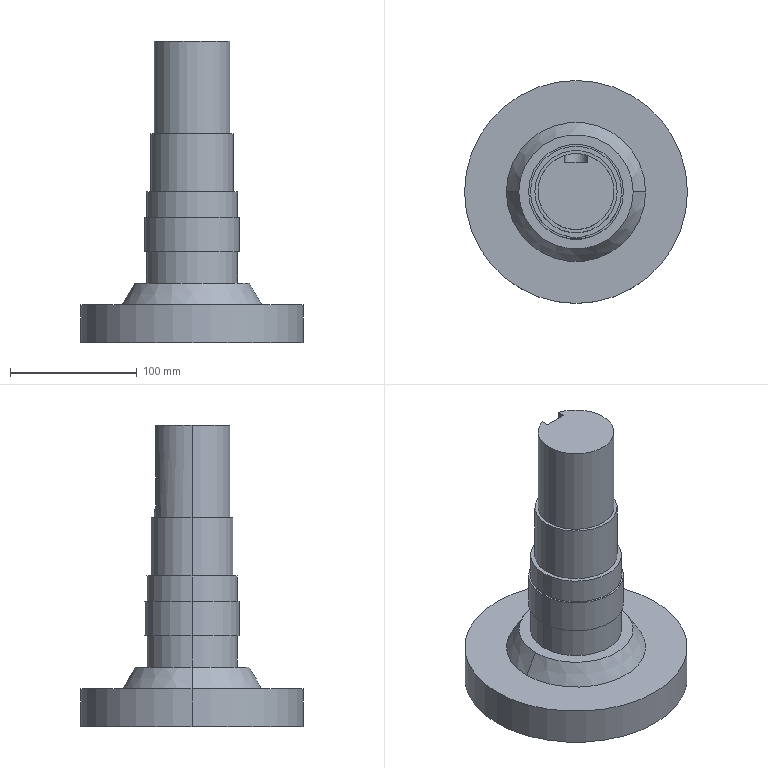Part | SolidWorks | features ICE 10, Chamfer 1, Extrusion 1, Fillet 1 | 1 solid | 37 faces | box 176 x 176 x 238 mm | volume 1296573 mm3 | cylinder 19 | plane 14 | torus 2 | cone 2 | commonest cylinder face diameters 72 x4 40 x2 60 x2 65 x2 75 x2 80 x2
STEP:
#1=CARTESIAN_POINT('',(-20.,0.,44.));
#2=VERTEX_POINT('',#1);
#3=CARTESIAN_POINT('',(20.,0.,44.));
#4=VERTEX_POINT('',#3);
#5=CARTESIAN_POINT('',(0.,0.,44.));
#6=DIRECTION('',(0.,0.,1.));
#7=DIRECTION('',(1.,0.,0.));
#8=AXIS2_PLACEMENT_3D('',#5,#6,#7);
#9=CIRCLE('',#8,20.);
#10=EDGE_CURVE('',#2,#4,#9,.T.);
#11=ORIENTED_EDGE('',*,*,#10,.T.);
#12=CARTESIAN_POINT('',(20.,0.,34.2));
#13=VERTEX_POINT('',#12);
#14=CARTESIAN_POINT('',(20.,0.,44.));
#15=DIRECTION('',(0.,0.,-1.));
#16=VECTOR('',#15,1000.);
#17=LINE('',#14,#16);
#18=EDGE_CURVE('',#4,#13,#17,.T.);
#19=ORIENTED_EDGE('',*,*,#18,.T.);
#20=CARTESIAN_POINT('',(-20.,0.,34.2));
#21=VERTEX_POINT('',#20);
#22=CARTESIAN_POINT('',(0.,0.,34.2));
#23=DIRECTION('',(0.,0.,1.));
#24=DIRECTION('',(-1.,0.,0.));
#25=AXIS2_PLACEMENT_3D('',#22,#23,#24);
#26=CIRCLE('',#25,20.);
#27=EDGE_CURVE('',#21,#13,#26,.T.);
#28=ORIENTED_EDGE('',*,*,#27,.F.);
#29=CARTESIAN_POINT('',(-20.,0.,44.));
#30=DIRECTION('',(0.,0.,-1.));
#31=VECTOR('',#30,1000.);
#32=LINE('',#29,#31);
#33=EDGE_CURVE('',#2,#21,#32,.T.);
#34=ORIENTED_EDGE('',*,*,#33,.F.);
#35=EDGE_LOOP('',(#11,#19,#28,#34));
#36=FACE_OUTER_BOUND('',#35,.T.);
#37=CARTESIAN_POINT('',(0.,0.,44.));
#38=DIRECTION('',(0.,0.,-1.));
#39=DIRECTION('',(-1.,0.,0.));
#40=AXIS2_PLACEMENT_3D('',#37,#38,#39);
#41=CYLINDRICAL_SURFACE('',#40,20.);
#42=ADVANCED_FACE('',(#36),#41,.F.);
#43=CARTESIAN_POINT('',(47.,0.,11.2));
#44=VERTEX_POINT('',#43);
#45=CARTESIAN_POINT('',(-47.,0.,11.2));
#46=VERTEX_POINT('',#45);
#47=CARTESIAN_POINT('',(0.,0.,11.2));
#48=DIRECTION('',(0.,0.,-1.));
#49=DIRECTION('',(-1.,0.,0.));
#50=AXIS2_PLACEMENT_3D('',#47,#48,#49);
#51=CIRCLE('',#50,47.);
#52=EDGE_CURVE('',#44,#46,#51,.T.);
#53=ORIENTED_EDGE('',*,*,#52,.F.);
#54=CARTESIAN_POINT('',(52.,0.,6.2));
#55=VERTEX_POINT('',#54);
#56=CARTESIAN_POINT('',(47.,0.,6.2));
#57=DIRECTION('',(0.,1.,0.));
#58=DIRECTION('',(-1.,0.,0.));
#59=AXIS2_PLACEMENT_3D('',#56,#57,#58);
#60=CIRCLE('',#59,5.);
#61=EDGE_CURVE('',#44,#55,#60,.T.);
#62=ORIENTED_EDGE('',*,*,#61,.T.);
#63=CARTESIAN_POINT('',(-52.,0.,6.2));
#64=VERTEX_POINT('',#63);
#65=CARTESIAN_POINT('',(0.,0.,6.2));
#66=DIRECTION('',(0.,0.,1.));
#67=DIRECTION('',(-1.,0.,0.));
#68=AXIS2_PLACEMENT_3D('',#65,#66,#67);
#69=CIRCLE('',#68,52.);
#70=EDGE_CURVE('',#64,#55,#69,.T.);
#71=ORIENTED_EDGE('',*,*,#70,.F.);
#72=CARTESIAN_POINT('',(-47.,0.,6.2));
#73=DIRECTION('',(0.,-1.,0.));
#74=DIRECTION('',(0.,0.,-1.));
#75=AXIS2_PLACEMENT_3D('',#72,#73,#74);
#76=CIRCLE('',#75,5.);
#77=EDGE_CURVE('',#46,#64,#76,.T.);
#78=ORIENTED_EDGE('',*,*,#77,.F.);
#79=EDGE_LOOP('',(#53,#62,#71,#78));
#80=FACE_OUTER_BOUND('',#79,.T.);
#81=CARTESIAN_POINT('',(0.,0.,6.2));
#82=DIRECTION('',(0.,0.,-1.));
#83=DIRECTION('',(-1.,0.,0.));
#84=AXIS2_PLACEMENT_3D('',#81,#82,#83);
#85=TOROIDAL_SURFACE('',#84,47.,5.);
#86=ADVANCED_FACE('',(#80),#85,.F.);
#87=CARTESIAN_POINT('',(40.,0.,34.2));
#88=VERTEX_POINT('',#87);
#89=CARTESIAN_POINT('',(-40.,0.,34.2));
#90=VERTEX_POINT('',#89);
#91=CARTESIAN_POINT('',(0.,0.,34.2));
#92=DIRECTION('',(0.,0.,-1.));
#93=DIRECTION('',(-1.,0.,0.));
#94=AXIS2_PLACEMENT_3D('',#91,#92,#93);
#95=CIRCLE('',#94,40.);
#96=EDGE_CURVE('',#88,#90,#95,.T.);
#97=ORIENTED_EDGE('',*,*,#96,.F.);
#98=CARTESIAN_POINT('',(40.,0.,11.2));
#99=VERTEX_POINT('',#98);
#100=CARTESIAN_POINT('',(40.,0.,34.2));
#101=DIRECTION('',(0.,0.,-1.));
#102=VECTOR('',#101,1000.);
#103=LINE('',#100,#102);
#104=EDGE_CURVE('',#88,#99,#103,.T.);
#105=ORIENTED_EDGE('',*,*,#104,.T.);
#106=CARTESIAN_POINT('',(-40.,0.,11.2));
#107=VERTEX_POINT('',#106);
#108=CARTESIAN_POINT('',(0.,0.,11.2));
#109=DIRECTION('',(0.,0.,-1.));
#110=DIRECTION('',(-1.,0.,0.));
#111=AXIS2_PLACEMENT_3D('',#108,#109,#110);
#112=CIRCLE('',#111,40.);
#113=EDGE_CURVE('',#99,#107,#112,.T.);
#114=ORIENTED_EDGE('',*,*,#113,.T.);
#115=CARTESIAN_POINT('',(-40.,0.,34.2));
#116=DIRECTION('',(0.,0.,-1.));
#117=VECTOR('',#116,1000.);
#118=LINE('',#115,#117);
#119=EDGE_CURVE('',#90,#107,#118,.T.);
#120=ORIENTED_EDGE('',*,*,#119,.F.);
#121=EDGE_LOOP('',(#97,#105,#114,#120));
#122=FACE_OUTER_BOUND('',#121,.T.);
#123=CARTESIAN_POINT('',(0.,0.,34.2));
#124=DIRECTION('',(0.,0.,-1.));
#125=DIRECTION('',(-1.,0.,0.));
#126=AXIS2_PLACEMENT_3D('',#123,#124,#125);
#127=CYLINDRICAL_SURFACE('',#126,40.);
#128=ADVANCED_FACE('',(#122),#127,.F.);
#129=ORIENTED_EDGE('',*,*,#70,.T.);
#130=CARTESIAN_POINT('',(52.,0.,0.));
#131=VERTEX_POINT('',#130);
#132=CARTESIAN_POINT('',(52.,0.,11.2));
#133=DIRECTION('',(0.,0.,-1.));
#134=VECTOR('',#133,1000.);
#135=LINE('',#132,#134);
#136=EDGE_CURVE('',#55,#131,#135,.T.);
#137=ORIENTED_EDGE('',*,*,#136,.T.);
#138=CARTESIAN_POINT('',(-52.,0.,0.));
#139=VERTEX_POINT('',#138);
#140=CARTESIAN_POINT('',(0.,0.,0.));
#141=DIRECTION('',(0.,0.,-1.));
#142=DIRECTION('',(-1.,0.,0.));
#143=AXIS2_PLACEMENT_3D('',#140,#141,#142);
#144=CIRCLE('',#143,52.);
#145=EDGE_CURVE('',#131,#139,#144,.T.);
#146=ORIENTED_EDGE('',*,*,#145,.T.);
#147=CARTESIAN_POINT('',(-52.,0.,11.2));
#148=DIRECTION('',(0.,0.,-1.));
#149=VECTOR('',#148,1000.);
#150=LINE('',#147,#149);
#151=EDGE_CURVE('',#64,#139,#150,.T.);
#152=ORIENTED_EDGE('',*,*,#151,.F.);
#153=EDGE_LOOP('',(#129,#137,#146,#152));
#154=FACE_OUTER_BOUND('',#153,.T.);
#155=CARTESIAN_POINT('',(0.,0.,11.2));
#156=DIRECTION('',(0.,0.,-1.));
#157=DIRECTION('',(-1.,0.,0.));
#158=AXIS2_PLACEMENT_3D('',#155,#156,#157);
#159=CYLINDRICAL_SURFACE('',#158,52.);
#160=ADVANCED_FACE('',(#154),#159,.F.);
#161=CARTESIAN_POINT('',(30.,0.,238.));
#162=VERTEX_POINT('',#161);
#163=CARTESIAN_POINT('',(9.,28.618,238.));
#164=VERTEX_POINT('',#163);
#165=CARTESIAN_POINT('',(0.,0.,238.));
#166=DIRECTION('',(0.,0.,1.));
#167=DIRECTION('',(1.,0.,0.));
#168=AXIS2_PLACEMENT_3D('',#165,#166,#167);
#169=CIRCLE('',#168,30.);
#170=EDGE_CURVE('',#162,#164,#169,.T.);
#171=ORIENTED_EDGE('',*,*,#170,.F.);
#172=CARTESIAN_POINT('',(30.,0.,165.));
#173=VERTEX_POINT('',#172);
#174=CARTESIAN_POINT('',(30.,0.,238.));
#175=DIRECTION('',(0.,0.,-1.));
#176=VECTOR('',#175,1000.);
#177=LINE('',#174,#176);
#178=EDGE_CURVE('',#162,#173,#177,.T.);
#179=ORIENTED_EDGE('',*,*,#178,.T.);
#180=CARTESIAN_POINT('',(-30.,0.,165.));
#181=VERTEX_POINT('',#180);
#182=CARTESIAN_POINT('',(0.,0.,165.));
#183=DIRECTION('',(0.,0.,-1.));
#184=DIRECTION('',(1.,0.,0.));
#185=AXIS2_PLACEMENT_3D('',#182,#183,#184);
#186=CIRCLE('',#185,30.);
#187=EDGE_CURVE('',#181,#173,#186,.T.);
#188=ORIENTED_EDGE('',*,*,#187,.F.);
#189=CARTESIAN_POINT('',(-30.,0.,238.));
#190=VERTEX_POINT('',#189);
#191=CARTESIAN_POINT('',(-30.,0.,238.));
#192=DIRECTION('',(0.,0.,-1.));
#193=VECTOR('',#192,1000.);
#194=LINE('',#191,#193);
#195=EDGE_CURVE('',#190,#181,#194,.T.);
#196=ORIENTED_EDGE('',*,*,#195,.F.);
#197=CARTESIAN_POINT('',(-9.,28.618,238.));
#198=VERTEX_POINT('',#197);
#199=CARTESIAN_POINT('',(0.,0.,238.));
#200=DIRECTION('',(0.,0.,1.));
#201=DIRECTION('',(1.,0.,0.));
#202=AXIS2_PLACEMENT_3D('',#199,#200,#201);
#203=CIRCLE('',#202,30.);
#204=EDGE_CURVE('',#198,#190,#203,.T.);
#205=ORIENTED_EDGE('',*,*,#204,.F.);
#206=CARTESIAN_POINT('',(-9.,28.618,178.));
#207=VERTEX_POINT('',#206);
#208=CARTESIAN_POINT('',(-9.,28.618,238.));
#209=DIRECTION('',(0.,0.,-1.));
#210=VECTOR('',#209,1000.);
#211=LINE('',#208,#210);
#212=EDGE_CURVE('',#198,#207,#211,.T.);
#213=ORIENTED_EDGE('',*,*,#212,.T.);
#214=CARTESIAN_POINT('',(9.,28.618,178.));
#215=VERTEX_POINT('',#214);
#216=CARTESIAN_POINT('',(-9.,28.618,178.));
#217=CARTESIAN_POINT('',(-9.,28.618,177.402));
#218=CARTESIAN_POINT('',(-8.941,28.637,176.814));
#219=CARTESIAN_POINT('',(-8.768,28.69,175.948));
#220=CARTESIAN_POINT('',(-8.696,28.712,175.662));
#221=CARTESIAN_POINT('',(-8.524,28.764,175.095));
#222=CARTESIAN_POINT('',(-8.423,28.794,174.815));
#223=CARTESIAN_POINT('',(-8.083,28.892,173.999));
#224=CARTESIAN_POINT('',(-7.807,28.968,173.483));
#225=CARTESIAN_POINT('',(-7.317,29.094,172.752));
#226=CARTESIAN_POINT('',(-7.14,29.138,172.514));
#227=CARTESIAN_POINT('',(-6.767,29.227,172.059));
#228=CARTESIAN_POINT('',(-6.571,29.272,171.843));
#229=CARTESIAN_POINT('',(-5.952,29.407,171.224));
#230=CARTESIAN_POINT('',(-5.501,29.495,170.853));
#231=CARTESIAN_POINT('',(-4.519,29.662,170.194));
#232=CARTESIAN_POINT('',(-4.001,29.737,169.917));
#233=CARTESIAN_POINT('',(-3.19,29.831,169.579));
#234=CARTESIAN_POINT('',(-2.914,29.86,169.48));
#235=CARTESIAN_POINT('',(-2.349,29.909,169.307));
#236=CARTESIAN_POINT('',(-2.058,29.931,169.233));
#237=CARTESIAN_POINT('',(-1.186,29.982,169.059));
#238=CARTESIAN_POINT('',(-0.5996,30.,169.001));
#239=CARTESIAN_POINT('',(0.5819,30.,168.999));
#240=CARTESIAN_POINT('',(1.182,29.982,169.058));
#241=CARTESIAN_POINT('',(2.339,29.914,169.289));
#242=CARTESIAN_POINT('',(2.902,29.864,169.46));
#243=CARTESIAN_POINT('',(3.723,29.769,169.801));
#244=CARTESIAN_POINT('',(3.991,29.734,169.928));
#245=CARTESIAN_POINT('',(4.509,29.66,170.206));
#246=CARTESIAN_POINT('',(4.76,29.621,170.356));
#247=CARTESIAN_POINT('',(5.246,29.539,170.681));
#248=CARTESIAN_POINT('',(5.481,29.496,170.855));
#249=CARTESIAN_POINT('',(5.934,29.408,171.227));
#250=CARTESIAN_POINT('',(6.154,29.363,171.426));
#251=CARTESIAN_POINT('',(6.777,29.228,172.049));
#252=CARTESIAN_POINT('',(7.148,29.138,172.5));
#253=CARTESIAN_POINT('',(7.799,28.97,173.471));
#254=CARTESIAN_POINT('',(8.082,28.892,173.997));
#255=CARTESIAN_POINT('',(8.534,28.762,175.081));
#256=CARTESIAN_POINT('',(8.706,28.709,175.642));
#257=CARTESIAN_POINT('',(8.881,28.655,176.513));
#258=CARTESIAN_POINT('',(8.926,28.641,176.81));
#259=CARTESIAN_POINT('',(8.985,28.623,177.403));
#260=CARTESIAN_POINT('',(9.,28.618,177.701));
#261=CARTESIAN_POINT('',(9.,28.618,178.));
#262=B_SPLINE_CURVE_WITH_KNOTS('',3,(#216,#217,#218,#219,#220,#221,#222,#223,#224,#225,#226,#227,#228,#229,#230,#231,#232,#233,#234,#235,#236,#237,#238,#239,#240,#241,#242,#243,#244,#245,#246,#247,#248,#249,#250,#251,#252,#253,#254,#255,#256,#257,#258,#259,#260,#261),.UNSPECIFIED.,.F.,.F.,(4,2,2,2,2,2,2,2,2,2,2,2,2,2,2,2,2,2,2,2,2,2,4),(0.,0.001768,0.002652,0.003536,0.005305,0.006189,0.007073,0.008841,0.01061,0.01149,0.01238,0.01415,0.01591,0.01768,0.01857,0.01945,0.02033,0.02122,0.02299,0.02476,0.02652,0.02741,0.02829),.UNSPECIFIED.);
#263=EDGE_CURVE('',#207,#215,#262,.T.);
#264=ORIENTED_EDGE('',*,*,#263,.T.);
#265=CARTESIAN_POINT('',(9.,28.618,238.));
#266=DIRECTION('',(0.,0.,1.));
#267=VECTOR('',#266,1000.);
#268=LINE('',#265,#267);
#269=EDGE_CURVE('',#215,#164,#268,.T.);
#270=ORIENTED_EDGE('',*,*,#269,.T.);
#271=EDGE_LOOP('',(#171,#179,#188,#196,#205,#213,#264,#270));
#272=FACE_OUTER_BOUND('',#271,.T.);
#273=CARTESIAN_POINT('',(0.,0.,238.));
#274=DIRECTION('',(0.,0.,-1.));
#275=DIRECTION('',(-1.,0.,0.));
#276=AXIS2_PLACEMENT_3D('',#273,#274,#275);
#277=CYLINDRICAL_SURFACE('',#276,30.);
#278=ADVANCED_FACE('',(#272),#277,.T.);
#279=CARTESIAN_POINT('',(32.5,0.,165.));
#280=VERTEX_POINT('',#279);
#281=CARTESIAN_POINT('',(-32.5,0.,165.));
#282=VERTEX_POINT('',#281);
#283=CARTESIAN_POINT('',(0.,0.,165.));
#284=DIRECTION('',(0.,0.,1.));
#285=DIRECTION('',(1.,0.,0.));
#286=AXIS2_PLACEMENT_3D('',#283,#284,#285);
#287=CIRCLE('',#286,32.5);
#288=EDGE_CURVE('',#280,#282,#287,.T.);
#289=ORIENTED_EDGE('',*,*,#288,.F.);
#290=CARTESIAN_POINT('',(32.5,0.,119.));
#291=VERTEX_POINT('',#290);
#292=CARTESIAN_POINT('',(32.5,0.,165.));
#293=DIRECTION('',(0.,0.,-1.));
#294=VECTOR('',#293,1000.);
#295=LINE('',#292,#294);
#296=EDGE_CURVE('',#280,#291,#295,.T.);
#297=ORIENTED_EDGE('',*,*,#296,.T.);
#298=CARTESIAN_POINT('',(-32.5,0.,119.));
#299=VERTEX_POINT('',#298);
#300=CARTESIAN_POINT('',(0.,0.,119.));
#301=DIRECTION('',(0.,0.,1.));
#302=DIRECTION('',(1.,0.,0.));
#303=AXIS2_PLACEMENT_3D('',#300,#301,#302);
#304=CIRCLE('',#303,32.5);
#305=EDGE_CURVE('',#291,#299,#304,.T.);
#306=ORIENTED_EDGE('',*,*,#305,.T.);
#307=CARTESIAN_POINT('',(-32.5,0.,165.));
#308=DIRECTION('',(0.,0.,-1.));
#309=VECTOR('',#308,1000.);
#310=LINE('',#307,#309);
#311=EDGE_CURVE('',#282,#299,#310,.T.);
#312=ORIENTED_EDGE('',*,*,#311,.F.);
#313=EDGE_LOOP('',(#289,#297,#306,#312));
#314=FACE_OUTER_BOUND('',#313,.T.);
#315=CARTESIAN_POINT('',(0.,0.,165.));
#316=DIRECTION('',(0.,0.,-1.));
#317=DIRECTION('',(-1.,0.,0.));
#318=AXIS2_PLACEMENT_3D('',#315,#316,#317);
#319=CYLINDRICAL_SURFACE('',#318,32.5);
#320=ADVANCED_FACE('',(#314),#319,.T.);
#321=CARTESIAN_POINT('',(36.,0.,119.));
#322=VERTEX_POINT('',#321);
#323=CARTESIAN_POINT('',(-36.,0.,119.));
#324=VERTEX_POINT('',#323);
#325=CARTESIAN_POINT('',(0.,0.,119.));
#326=DIRECTION('',(0.,0.,1.));
#327=DIRECTION('',(1.,0.,0.));
#328=AXIS2_PLACEMENT_3D('',#325,#326,#327);
#329=CIRCLE('',#328,36.);
#330=EDGE_CURVE('',#322,#324,#329,.T.);
#331=ORIENTED_EDGE('',*,*,#330,.F.);
#332=CARTESIAN_POINT('',(36.,0.,99.));
#333=VERTEX_POINT('',#332);
#334=CARTESIAN_POINT('',(36.,0.,119.));
#335=DIRECTION('',(0.,0.,-1.));
#336=VECTOR('',#335,1000.);
#337=LINE('',#334,#336);
#338=EDGE_CURVE('',#322,#333,#337,.T.);
#339=ORIENTED_EDGE('',*,*,#338,.T.);
#340=CARTESIAN_POINT('',(-36.,0.,99.));
#341=VERTEX_POINT('',#340);
#342=CARTESIAN_POINT('',(0.,0.,99.));
#343=DIRECTION('',(0.,0.,1.));
#344=DIRECTION('',(1.,0.,0.));
#345=AXIS2_PLACEMENT_3D('',#342,#343,#344);
#346=CIRCLE('',#345,36.);
#347=EDGE_CURVE('',#333,#341,#346,.T.);
#348=ORIENTED_EDGE('',*,*,#347,.T.);
#349=CARTESIAN_POINT('',(-36.,0.,119.));
#350=DIRECTION('',(0.,0.,-1.));
#351=VECTOR('',#350,1000.);
#352=LINE('',#349,#351);
#353=EDGE_CURVE('',#324,#341,#352,.T.);
#354=ORIENTED_EDGE('',*,*,#353,.F.);
#355=EDGE_LOOP('',(#331,#339,#348,#354));
#356=FACE_OUTER_BOUND('',#355,.T.);
#357=CARTESIAN_POINT('',(0.,0.,119.));
#358=DIRECTION('',(0.,0.,-1.));
#359=DIRECTION('',(-1.,0.,0.));
#360=AXIS2_PLACEMENT_3D('',#357,#358,#359);
#361=CYLINDRICAL_SURFACE('',#360,36.);
#362=ADVANCED_FACE('',(#356),#361,.T.);
#363=CARTESIAN_POINT('',(37.5,0.,99.));
#364=VERTEX_POINT('',#363);
#365=CARTESIAN_POINT('',(-37.5,0.,99.));
#366=VERTEX_POINT('',#365);
#367=CARTESIAN_POINT('',(0.,0.,99.));
#368=DIRECTION('',(0.,0.,1.));
#369=DIRECTION('',(1.,0.,0.));
#370=AXIS2_PLACEMENT_3D('',#367,#368,#369);
#371=CIRCLE('',#370,37.5);
#372=EDGE_CURVE('',#364,#366,#371,.T.);
#373=ORIENTED_EDGE('',*,*,#372,.F.);
#374=CARTESIAN_POINT('',(37.5,0.,72.));
#375=VERTEX_POINT('',#374);
#376=CARTESIAN_POINT('',(37.5,0.,99.));
#377=DIRECTION('',(0.,0.,-1.));
#378=VECTOR('',#377,1000.);
#379=LINE('',#376,#378);
#380=EDGE_CURVE('',#364,#375,#379,.T.);
#381=ORIENTED_EDGE('',*,*,#380,.T.);
#382=CARTESIAN_POINT('',(-37.5,0.,72.));
#383=VERTEX_POINT('',#382);
#384=CARTESIAN_POINT('',(0.,0.,72.));
#385=DIRECTION('',(0.,0.,1.));
#386=DIRECTION('',(1.,0.,0.));
#387=AXIS2_PLACEMENT_3D('',#384,#385,#386);
#388=CIRCLE('',#387,37.5);
#389=EDGE_CURVE('',#375,#383,#388,.T.);
#390=ORIENTED_EDGE('',*,*,#389,.T.);
#391=CARTESIAN_POINT('',(-37.5,0.,99.));
#392=DIRECTION('',(0.,0.,-1.));
#393=VECTOR('',#392,1000.);
#394=LINE('',#391,#393);
#395=EDGE_CURVE('',#366,#383,#394,.T.);
#396=ORIENTED_EDGE('',*,*,#395,.F.);
#397=EDGE_LOOP('',(#373,#381,#390,#396));
#398=FACE_OUTER_BOUND('',#397,.T.);
#399=CARTESIAN_POINT('',(0.,0.,99.));
#400=DIRECTION('',(0.,0.,-1.));
#401=DIRECTION('',(-1.,0.,0.));
#402=AXIS2_PLACEMENT_3D('',#399,#400,#401);
#403=CYLINDRICAL_SURFACE('',#402,37.5);
#404=ADVANCED_FACE('',(#398),#403,.T.);
#405=CARTESIAN_POINT('',(36.,0.,72.));
#406=VERTEX_POINT('',#405);
#407=CARTESIAN_POINT('',(-36.,0.,72.));
#408=VERTEX_POINT('',#407);
#409=CARTESIAN_POINT('',(0.,0.,72.));
#410=DIRECTION('',(0.,0.,1.));
#411=DIRECTION('',(1.,0.,0.));
#412=AXIS2_PLACEMENT_3D('',#409,#410,#411);
#413=CIRCLE('',#412,36.);
#414=EDGE_CURVE('',#406,#408,#413,.T.);
#415=ORIENTED_EDGE('',*,*,#414,.F.);
#416=CARTESIAN_POINT('',(36.,0.,47.));
#417=VERTEX_POINT('',#416);
#418=CARTESIAN_POINT('',(36.,0.,72.));
#419=DIRECTION('',(0.,0.,-1.));
#420=VECTOR('',#419,1000.);
#421=LINE('',#418,#420);
#422=EDGE_CURVE('',#406,#417,#421,.T.);
#423=ORIENTED_EDGE('',*,*,#422,.T.);
#424=CARTESIAN_POINT('',(-36.,0.,47.));
#425=VERTEX_POINT('',#424);
#426=CARTESIAN_POINT('',(0.,0.,47.));
#427=DIRECTION('',(0.,0.,1.));
#428=DIRECTION('',(1.,0.,0.));
#429=AXIS2_PLACEMENT_3D('',#426,#427,#428);
#430=CIRCLE('',#429,36.);
#431=EDGE_CURVE('',#417,#425,#430,.T.);
#432=ORIENTED_EDGE('',*,*,#431,.T.);
#433=CARTESIAN_POINT('',(-36.,0.,72.));
#434=DIRECTION('',(0.,0.,-1.));
#435=VECTOR('',#434,1000.);
#436=LINE('',#433,#435);
#437=EDGE_CURVE('',#408,#425,#436,.T.);
#438=ORIENTED_EDGE('',*,*,#437,.F.);
#439=EDGE_LOOP('',(#415,#423,#432,#438));
#440=FACE_OUTER_BOUND('',#439,.T.);
#441=CARTESIAN_POINT('',(0.,0.,72.));
#442=DIRECTION('',(0.,0.,-1.));
#443=DIRECTION('',(-1.,0.,0.));
#444=AXIS2_PLACEMENT_3D('',#441,#442,#443);
#445=CYLINDRICAL_SURFACE('',#444,36.);
#446=ADVANCED_FACE('',(#440),#445,.T.);
#447=CARTESIAN_POINT('',(45.185,0.,47.));
#448=VERTEX_POINT('',#447);
#449=CARTESIAN_POINT('',(-45.185,0.,47.));
#450=VERTEX_POINT('',#449);
#451=CARTESIAN_POINT('',(0.,0.,47.));
#452=DIRECTION('',(0.,0.,1.));
#453=DIRECTION('',(1.,0.,0.));
#454=AXIS2_PLACEMENT_3D('',#451,#452,#453);
#455=CIRCLE('',#454,45.185);
#456=EDGE_CURVE('',#448,#450,#455,.T.);
#457=ORIENTED_EDGE('',*,*,#456,.F.);
#458=CARTESIAN_POINT('',(55.,0.,30.));
#459=VERTEX_POINT('',#458);
#460=CARTESIAN_POINT('',(45.185,0.,47.));
#461=DIRECTION('',(0.5,0.,-0.866));
#462=VECTOR('',#461,1000.);
#463=LINE('',#460,#462);
#464=EDGE_CURVE('',#448,#459,#463,.T.);
#465=ORIENTED_EDGE('',*,*,#464,.T.);
#466=CARTESIAN_POINT('',(-55.,0.,30.));
#467=VERTEX_POINT('',#466);
#468=CARTESIAN_POINT('',(0.,0.,30.));
#469=DIRECTION('',(0.,0.,1.));
#470=DIRECTION('',(1.,0.,0.));
#471=AXIS2_PLACEMENT_3D('',#468,#469,#470);
#472=CIRCLE('',#471,55.);
#473=EDGE_CURVE('',#459,#467,#472,.T.);
#474=ORIENTED_EDGE('',*,*,#473,.T.);
#475=CARTESIAN_POINT('',(-45.185,0.,47.));
#476=DIRECTION('',(-0.5,0.,-0.866));
#477=VECTOR('',#476,1000.);
#478=LINE('',#475,#477);
#479=EDGE_CURVE('',#450,#467,#478,.T.);
#480=ORIENTED_EDGE('',*,*,#479,.F.);
#481=EDGE_LOOP('',(#457,#465,#474,#480));
#482=FACE_OUTER_BOUND('',#481,.T.);
#483=CARTESIAN_POINT('',(0.,0.,47.));
#484=DIRECTION('',(0.,0.,-1.));
#485=DIRECTION('',(-1.,0.,0.));
#486=AXIS2_PLACEMENT_3D('',#483,#484,#485);
#487=CONICAL_SURFACE('',#486,45.185,0.5236);
#488=ADVANCED_FACE('',(#482),#487,.T.);
#489=CARTESIAN_POINT('',(88.,0.,30.));
#490=VERTEX_POINT('',#489);
#491=CARTESIAN_POINT('',(-88.,0.,30.));
#492=VERTEX_POINT('',#491);
#493=CARTESIAN_POINT('',(0.,0.,30.));
#494=DIRECTION('',(0.,0.,1.));
#495=DIRECTION('',(1.,0.,0.));
#496=AXIS2_PLACEMENT_3D('',#493,#494,#495);
#497=CIRCLE('',#496,88.);
#498=EDGE_CURVE('',#490,#492,#497,.T.);
#499=ORIENTED_EDGE('',*,*,#498,.F.);
#500=CARTESIAN_POINT('',(88.,0.,0.));
#501=VERTEX_POINT('',#500);
#502=CARTESIAN_POINT('',(88.,0.,30.));
#503=DIRECTION('',(0.,0.,-1.));
#504=VECTOR('',#503,1000.);
#505=LINE('',#502,#504);
#506=EDGE_CURVE('',#490,#501,#505,.T.);
#507=ORIENTED_EDGE('',*,*,#506,.T.);
#508=CARTESIAN_POINT('',(-88.,0.,0.));
#509=VERTEX_POINT('',#508);
#510=CARTESIAN_POINT('',(0.,0.,0.));
#511=DIRECTION('',(0.,0.,1.));
#512=DIRECTION('',(1.,0.,0.));
#513=AXIS2_PLACEMENT_3D('',#510,#511,#512);
#514=CIRCLE('',#513,88.);
#515=EDGE_CURVE('',#501,#509,#514,.T.);
#516=ORIENTED_EDGE('',*,*,#515,.T.);
#517=CARTESIAN_POINT('',(-88.,0.,30.));
#518=DIRECTION('',(0.,0.,-1.));
#519=VECTOR('',#518,1000.);
#520=LINE('',#517,#519);
#521=EDGE_CURVE('',#492,#509,#520,.T.);
#522=ORIENTED_EDGE('',*,*,#521,.F.);
#523=EDGE_LOOP('',(#499,#507,#516,#522));
#524=FACE_OUTER_BOUND('',#523,.T.);
#525=CARTESIAN_POINT('',(0.,0.,30.));
#526=DIRECTION('',(0.,0.,-1.));
#527=DIRECTION('',(-1.,0.,0.));
#528=AXIS2_PLACEMENT_3D('',#525,#526,#527);
#529=CYLINDRICAL_SURFACE('',#528,88.);
#530=ADVANCED_FACE('',(#524),#529,.T.);
#531=ORIENTED_EDGE('',*,*,#506,.F.);
#532=CARTESIAN_POINT('',(0.,0.,30.));
#533=DIRECTION('',(0.,0.,1.));
#534=DIRECTION('',(1.,0.,0.));
#535=AXIS2_PLACEMENT_3D('',#532,#533,#534);
#536=CIRCLE('',#535,88.);
#537=EDGE_CURVE('',#492,#490,#536,.T.);
#538=ORIENTED_EDGE('',*,*,#537,.F.);
#539=ORIENTED_EDGE('',*,*,#521,.T.);
#540=CARTESIAN_POINT('',(0.,0.,0.));
#541=DIRECTION('',(0.,0.,1.));
#542=DIRECTION('',(1.,0.,0.));
#543=AXIS2_PLACEMENT_3D('',#540,#541,#542);
#544=CIRCLE('',#543,88.);
#545=EDGE_CURVE('',#509,#501,#544,.T.);
#546=ORIENTED_EDGE('',*,*,#545,.T.);
#547=EDGE_LOOP('',(#531,#538,#539,#546));
#548=FACE_OUTER_BOUND('',#547,.T.);
#549=CARTESIAN_POINT('',(0.,0.,30.));
#550=DIRECTION('',(0.,0.,-1.));
#551=DIRECTION('',(-1.,0.,0.));
#552=AXIS2_PLACEMENT_3D('',#549,#550,#551);
#553=CYLINDRICAL_SURFACE('',#552,88.);
#554=ADVANCED_FACE('',(#548),#553,.T.);
#555=CARTESIAN_POINT('',(0.,0.,30.));
#556=DIRECTION('',(0.,0.,1.));
#557=DIRECTION('',(1.,0.,0.));
#558=AXIS2_PLACEMENT_3D('',#555,#556,#557);
#559=CIRCLE('',#558,55.);
#560=EDGE_CURVE('',#467,#459,#559,.T.);
#561=ORIENTED_EDGE('',*,*,#560,.F.);
#562=ORIENTED_EDGE('',*,*,#473,.F.);
#563=EDGE_LOOP('',(#561,#562));
#564=FACE_BOUND('',#563,.T.);
#565=ORIENTED_EDGE('',*,*,#537,.T.);
#566=ORIENTED_EDGE('',*,*,#498,.T.);
#567=EDGE_LOOP('',(#565,#566));
#568=FACE_OUTER_BOUND('',#567,.T.);
#569=CARTESIAN_POINT('',(0.,0.,30.));
#570=DIRECTION('',(0.,0.,1.));
#571=DIRECTION('',(1.,0.,0.));
#572=AXIS2_PLACEMENT_3D('',#569,#570,#571);
#573=PLANE('',#572);
#574=ADVANCED_FACE('',(#564,#568),#573,.T.);
#575=CARTESIAN_POINT('',(0.,0.,0.));
#576=DIRECTION('',(0.,0.,-1.));
#577=DIRECTION('',(-1.,0.,0.));
#578=AXIS2_PLACEMENT_3D('',#575,#576,#577);
#579=CIRCLE('',#578,52.);
#580=EDGE_CURVE('',#139,#131,#579,.T.);
#581=ORIENTED_EDGE('',*,*,#580,.F.);
#582=ORIENTED_EDGE('',*,*,#145,.F.);
#583=EDGE_LOOP('',(#581,#582));
#584=FACE_BOUND('',#583,.T.);
#585=ORIENTED_EDGE('',*,*,#545,.F.);
#586=ORIENTED_EDGE('',*,*,#515,.F.);
#587=EDGE_LOOP('',(#585,#586));
#588=FACE_OUTER_BOUND('',#587,.T.);
#589=CARTESIAN_POINT('',(0.,0.,0.));
#590=DIRECTION('',(0.,0.,1.));
#591=DIRECTION('',(1.,0.,0.));
#592=AXIS2_PLACEMENT_3D('',#589,#590,#591);
#593=PLANE('',#592);
#594=ADVANCED_FACE('',(#584,#588),#593,.F.);
#595=CARTESIAN_POINT('',(0.,0.,47.));
#596=DIRECTION('',(0.,0.,1.));
#597=DIRECTION('',(1.,0.,0.));
#598=AXIS2_PLACEMENT_3D('',#595,#596,#597);
#599=CIRCLE('',#598,36.);
#600=EDGE_CURVE('',#425,#417,#599,.T.);
#601=ORIENTED_EDGE('',*,*,#600,.F.);
#602=ORIENTED_EDGE('',*,*,#431,.F.);
#603=EDGE_LOOP('',(#601,#602));
#604=FACE_BOUND('',#603,.T.);
#605=CARTESIAN_POINT('',(0.,0.,47.));
#606=DIRECTION('',(0.,0.,1.));
#607=DIRECTION('',(1.,0.,0.));
#608=AXIS2_PLACEMENT_3D('',#605,#606,#607);
#609=CIRCLE('',#608,45.185);
#610=EDGE_CURVE('',#450,#448,#609,.T.);
#611=ORIENTED_EDGE('',*,*,#610,.T.);
#612=ORIENTED_EDGE('',*,*,#456,.T.);
#613=EDGE_LOOP('',(#611,#612));
#614=FACE_OUTER_BOUND('',#613,.T.);
#615=CARTESIAN_POINT('',(0.,0.,47.));
#616=DIRECTION('',(0.,0.,1.));
#617=DIRECTION('',(1.,0.,0.));
#618=AXIS2_PLACEMENT_3D('',#615,#616,#617);
#619=PLANE('',#618);
#620=ADVANCED_FACE('',(#604,#614),#619,.T.);
#621=ORIENTED_EDGE('',*,*,#464,.F.);
#622=ORIENTED_EDGE('',*,*,#610,.F.);
#623=ORIENTED_EDGE('',*,*,#479,.T.);
#624=ORIENTED_EDGE('',*,*,#560,.T.);
#625=EDGE_LOOP('',(#621,#622,#623,#624));
#626=FACE_OUTER_BOUND('',#625,.T.);
#627=CARTESIAN_POINT('',(0.,0.,47.));
#628=DIRECTION('',(0.,0.,-1.));
#629=DIRECTION('',(-1.,0.,0.));
#630=AXIS2_PLACEMENT_3D('',#627,#628,#629);
#631=CONICAL_SURFACE('',#630,45.185,0.5236);
#632=ADVANCED_FACE('',(#626),#631,.T.);
#633=ORIENTED_EDGE('',*,*,#422,.F.);
#634=CARTESIAN_POINT('',(0.,0.,72.));
#635=DIRECTION('',(0.,0.,1.));
#636=DIRECTION('',(1.,0.,0.));
#637=AXIS2_PLACEMENT_3D('',#634,#635,#636);
#638=CIRCLE('',#637,36.);
#639=EDGE_CURVE('',#408,#406,#638,.T.);
#640=ORIENTED_EDGE('',*,*,#639,.F.);
#641=ORIENTED_EDGE('',*,*,#437,.T.);
#642=ORIENTED_EDGE('',*,*,#600,.T.);
#643=EDGE_LOOP('',(#633,#640,#641,#642));
#644=FACE_OUTER_BOUND('',#643,.T.);
#645=CARTESIAN_POINT('',(0.,0.,72.));
#646=DIRECTION('',(0.,0.,-1.));
#647=DIRECTION('',(-1.,0.,0.));
#648=AXIS2_PLACEMENT_3D('',#645,#646,#647);
#649=CYLINDRICAL_SURFACE('',#648,36.);
#650=ADVANCED_FACE('',(#644),#649,.T.);
#651=ORIENTED_EDGE('',*,*,#380,.F.);
#652=CARTESIAN_POINT('',(0.,0.,99.));
#653=DIRECTION('',(0.,0.,1.));
#654=DIRECTION('',(1.,0.,0.));
#655=AXIS2_PLACEMENT_3D('',#652,#653,#654);
#656=CIRCLE('',#655,37.5);
#657=EDGE_CURVE('',#366,#364,#656,.T.);
#658=ORIENTED_EDGE('',*,*,#657,.F.);
#659=ORIENTED_EDGE('',*,*,#395,.T.);
#660=CARTESIAN_POINT('',(0.,0.,72.));
#661=DIRECTION('',(0.,0.,1.));
#662=DIRECTION('',(1.,0.,0.));
#663=AXIS2_PLACEMENT_3D('',#660,#661,#662);
#664=CIRCLE('',#663,37.5);
#665=EDGE_CURVE('',#383,#375,#664,.T.);
#666=ORIENTED_EDGE('',*,*,#665,.T.);
#667=EDGE_LOOP('',(#651,#658,#659,#666));
#668=FACE_OUTER_BOUND('',#667,.T.);
#669=CARTESIAN_POINT('',(0.,0.,99.));
#670=DIRECTION('',(0.,0.,-1.));
#671=DIRECTION('',(-1.,0.,0.));
#672=AXIS2_PLACEMENT_3D('',#669,#670,#671);
#673=CYLINDRICAL_SURFACE('',#672,37.5);
#674=ADVANCED_FACE('',(#668),#673,.T.);
#675=CARTESIAN_POINT('',(0.,0.,99.));
#676=DIRECTION('',(0.,0.,1.));
#677=DIRECTION('',(1.,0.,0.));
#678=AXIS2_PLACEMENT_3D('',#675,#676,#677);
#679=CIRCLE('',#678,36.);
#680=EDGE_CURVE('',#341,#333,#679,.T.);
#681=ORIENTED_EDGE('',*,*,#680,.F.);
#682=ORIENTED_EDGE('',*,*,#347,.F.);
#683=EDGE_LOOP('',(#681,#682));
#684=FACE_BOUND('',#683,.T.);
#685=ORIENTED_EDGE('',*,*,#657,.T.);
#686=ORIENTED_EDGE('',*,*,#372,.T.);
#687=EDGE_LOOP('',(#685,#686));
#688=FACE_OUTER_BOUND('',#687,.T.);
#689=CARTESIAN_POINT('',(0.,0.,99.));
#690=DIRECTION('',(0.,0.,1.));
#691=DIRECTION('',(1.,0.,0.));
#692=AXIS2_PLACEMENT_3D('',#689,#690,#691);
#693=PLANE('',#692);
#694=ADVANCED_FACE('',(#684,#688),#693,.T.);
#695=ORIENTED_EDGE('',*,*,#639,.T.);
#696=ORIENTED_EDGE('',*,*,#414,.T.);
#697=EDGE_LOOP('',(#695,#696));
#698=FACE_BOUND('',#697,.T.);
#699=ORIENTED_EDGE('',*,*,#665,.F.);
#700=ORIENTED_EDGE('',*,*,#389,.F.);
#701=EDGE_LOOP('',(#699,#700));
#702=FACE_OUTER_BOUND('',#701,.T.);
#703=CARTESIAN_POINT('',(0.,0.,72.));
#704=DIRECTION('',(0.,0.,1.));
#705=DIRECTION('',(1.,0.,0.));
#706=AXIS2_PLACEMENT_3D('',#703,#704,#705);
#707=PLANE('',#706);
#708=ADVANCED_FACE('',(#698,#702),#707,.F.);
#709=ORIENTED_EDGE('',*,*,#338,.F.);
#710=CARTESIAN_POINT('',(0.,0.,119.));
#711=DIRECTION('',(0.,0.,1.));
#712=DIRECTION('',(1.,0.,0.));
#713=AXIS2_PLACEMENT_3D('',#710,#711,#712);
#714=CIRCLE('',#713,36.);
#715=EDGE_CURVE('',#324,#322,#714,.T.);
#716=ORIENTED_EDGE('',*,*,#715,.F.);
#717=ORIENTED_EDGE('',*,*,#353,.T.);
#718=ORIENTED_EDGE('',*,*,#680,.T.);
#719=EDGE_LOOP('',(#709,#716,#717,#718));
#720=FACE_OUTER_BOUND('',#719,.T.);
#721=CARTESIAN_POINT('',(0.,0.,119.));
#722=DIRECTION('',(0.,0.,-1.));
#723=DIRECTION('',(-1.,0.,0.));
#724=AXIS2_PLACEMENT_3D('',#721,#722,#723);
#725=CYLINDRICAL_SURFACE('',#724,36.);
#726=ADVANCED_FACE('',(#720),#725,.T.);
#727=CARTESIAN_POINT('',(0.,0.,119.));
#728=DIRECTION('',(0.,0.,1.));
#729=DIRECTION('',(1.,0.,0.));
#730=AXIS2_PLACEMENT_3D('',#727,#728,#729);
#731=CIRCLE('',#730,32.5);
#732=EDGE_CURVE('',#299,#291,#731,.T.);
#733=ORIENTED_EDGE('',*,*,#732,.F.);
#734=ORIENTED_EDGE('',*,*,#305,.F.);
#735=EDGE_LOOP('',(#733,#734));
#736=FACE_BOUND('',#735,.T.);
#737=ORIENTED_EDGE('',*,*,#715,.T.);
#738=ORIENTED_EDGE('',*,*,#330,.T.);
#739=EDGE_LOOP('',(#737,#738));
#740=FACE_OUTER_BOUND('',#739,.T.);
#741=CARTESIAN_POINT('',(0.,0.,119.));
#742=DIRECTION('',(0.,0.,1.));
#743=DIRECTION('',(1.,0.,0.));
#744=AXIS2_PLACEMENT_3D('',#741,#742,#743);
#745=PLANE('',#744);
#746=ADVANCED_FACE('',(#736,#740),#745,.T.);
#747=ORIENTED_EDGE('',*,*,#296,.F.);
#748=CARTESIAN_POINT('',(0.,0.,165.));
#749=DIRECTION('',(0.,0.,1.));
#750=DIRECTION('',(1.,0.,0.));
#751=AXIS2_PLACEMENT_3D('',#748,#749,#750);
#752=CIRCLE('',#751,32.5);
#753=EDGE_CURVE('',#282,#280,#752,.T.);
#754=ORIENTED_EDGE('',*,*,#753,.F.);
#755=ORIENTED_EDGE('',*,*,#311,.T.);
#756=ORIENTED_EDGE('',*,*,#732,.T.);
#757=EDGE_LOOP('',(#747,#754,#755,#756));
#758=FACE_OUTER_BOUND('',#757,.T.);
#759=CARTESIAN_POINT('',(0.,0.,165.));
#760=DIRECTION('',(0.,0.,-1.));
#761=DIRECTION('',(-1.,0.,0.));
#762=AXIS2_PLACEMENT_3D('',#759,#760,#761);
#763=CYLINDRICAL_SURFACE('',#762,32.5);
#764=ADVANCED_FACE('',(#758),#763,.T.);
#765=ORIENTED_EDGE('',*,*,#187,.T.);
#766=CARTESIAN_POINT('',(0.,0.,165.));
#767=DIRECTION('',(0.,0.,-1.));
#768=DIRECTION('',(1.,0.,0.));
#769=AXIS2_PLACEMENT_3D('',#766,#767,#768);
#770=CIRCLE('',#769,30.);
#771=EDGE_CURVE('',#173,#181,#770,.T.);
#772=ORIENTED_EDGE('',*,*,#771,.T.);
#773=EDGE_LOOP('',(#765,#772));
#774=FACE_BOUND('',#773,.T.);
#775=ORIENTED_EDGE('',*,*,#753,.T.);
#776=ORIENTED_EDGE('',*,*,#288,.T.);
#777=EDGE_LOOP('',(#775,#776));
#778=FACE_OUTER_BOUND('',#777,.T.);
#779=CARTESIAN_POINT('',(0.,0.,165.));
#780=DIRECTION('',(0.,0.,1.));
#781=DIRECTION('',(1.,0.,0.));
#782=AXIS2_PLACEMENT_3D('',#779,#780,#781);
#783=PLANE('',#782);
#784=ADVANCED_FACE('',(#774,#778),#783,.T.);
#785=ORIENTED_EDGE('',*,*,#178,.F.);
#786=CARTESIAN_POINT('',(0.,0.,238.));
#787=DIRECTION('',(0.,0.,1.));
#788=DIRECTION('',(1.,0.,0.));
#789=AXIS2_PLACEMENT_3D('',#786,#787,#788);
#790=CIRCLE('',#789,30.);
#791=EDGE_CURVE('',#190,#162,#790,.T.);
#792=ORIENTED_EDGE('',*,*,#791,.F.);
#793=ORIENTED_EDGE('',*,*,#195,.T.);
#794=ORIENTED_EDGE('',*,*,#771,.F.);
#795=EDGE_LOOP('',(#785,#792,#793,#794));
#796=FACE_OUTER_BOUND('',#795,.T.);
#797=CARTESIAN_POINT('',(0.,0.,238.));
#798=DIRECTION('',(0.,0.,-1.));
#799=DIRECTION('',(-1.,0.,0.));
#800=AXIS2_PLACEMENT_3D('',#797,#798,#799);
#801=CYLINDRICAL_SURFACE('',#800,30.);
#802=ADVANCED_FACE('',(#796),#801,.T.);
#803=CARTESIAN_POINT('',(-9.,23.,238.));
#804=VERTEX_POINT('',#803);
#805=CARTESIAN_POINT('',(-9.,23.,238.));
#806=DIRECTION('',(0.,1.,0.));
#807=VECTOR('',#806,1000.);
#808=LINE('',#805,#807);
#809=EDGE_CURVE('',#804,#198,#808,.T.);
#810=ORIENTED_EDGE('',*,*,#809,.T.);
#811=ORIENTED_EDGE('',*,*,#204,.T.);
#812=ORIENTED_EDGE('',*,*,#791,.T.);
#813=ORIENTED_EDGE('',*,*,#170,.T.);
#814=CARTESIAN_POINT('',(9.,23.,238.));
#815=VERTEX_POINT('',#814);
#816=CARTESIAN_POINT('',(9.,23.,238.));
#817=DIRECTION('',(0.,1.,0.));
#818=VECTOR('',#817,1000.);
#819=LINE('',#816,#818);
#820=EDGE_CURVE('',#815,#164,#819,.T.);
#821=ORIENTED_EDGE('',*,*,#820,.F.);
#822=CARTESIAN_POINT('',(0.,23.,238.));
#823=DIRECTION('',(-1.,0.,0.));
#824=VECTOR('',#823,1000.);
#825=LINE('',#822,#824);
#826=EDGE_CURVE('',#815,#804,#825,.T.);
#827=ORIENTED_EDGE('',*,*,#826,.T.);
#828=EDGE_LOOP('',(#810,#811,#812,#813,#821,#827));
#829=FACE_OUTER_BOUND('',#828,.T.);
#830=CARTESIAN_POINT('',(0.,0.,238.));
#831=DIRECTION('',(0.,0.,1.));
#832=DIRECTION('',(1.,0.,0.));
#833=AXIS2_PLACEMENT_3D('',#830,#831,#832);
#834=PLANE('',#833);
#835=ADVANCED_FACE('',(#829),#834,.T.);
#836=CARTESIAN_POINT('',(-9.,23.,178.));
#837=VERTEX_POINT('',#836);
#838=CARTESIAN_POINT('',(-9.,23.,178.));
#839=DIRECTION('',(0.,1.,0.));
#840=VECTOR('',#839,1000.);
#841=LINE('',#838,#840);
#842=EDGE_CURVE('',#837,#207,#841,.T.);
#843=ORIENTED_EDGE('',*,*,#842,.F.);
#844=CARTESIAN_POINT('',(9.,23.,178.));
#845=VERTEX_POINT('',#844);
#846=CARTESIAN_POINT('',(0.,23.,178.));
#847=DIRECTION('',(0.,1.,0.));
#848=DIRECTION('',(0.,0.,1.));
#849=AXIS2_PLACEMENT_3D('',#846,#847,#848);
#850=CIRCLE('',#849,9.);
#851=EDGE_CURVE('',#845,#837,#850,.T.);
#852=ORIENTED_EDGE('',*,*,#851,.F.);
#853=CARTESIAN_POINT('',(9.,23.,178.));
#854=DIRECTION('',(0.,1.,0.));
#855=VECTOR('',#854,1000.);
#856=LINE('',#853,#855);
#857=EDGE_CURVE('',#845,#215,#856,.T.);
#858=ORIENTED_EDGE('',*,*,#857,.T.);
#859=ORIENTED_EDGE('',*,*,#263,.F.);
#860=EDGE_LOOP('',(#843,#852,#858,#859));
#861=FACE_OUTER_BOUND('',#860,.T.);
#862=CARTESIAN_POINT('',(0.,23.,178.));
#863=DIRECTION('',(0.,1.,0.));
#864=DIRECTION('',(0.,0.,1.));
#865=AXIS2_PLACEMENT_3D('',#862,#863,#864);
#866=CYLINDRICAL_SURFACE('',#865,9.);
#867=ADVANCED_FACE('',(#861),#866,.F.);
#868=ORIENTED_EDGE('',*,*,#809,.F.);
#869=CARTESIAN_POINT('',(-9.,23.,238.));
#870=DIRECTION('',(0.,0.,1.));
#871=VECTOR('',#870,1000.);
#872=LINE('',#869,#871);
#873=EDGE_CURVE('',#837,#804,#872,.T.);
#874=ORIENTED_EDGE('',*,*,#873,.F.);
#875=ORIENTED_EDGE('',*,*,#842,.T.);
#876=ORIENTED_EDGE('',*,*,#212,.F.);
#877=EDGE_LOOP('',(#868,#874,#875,#876));
#878=FACE_OUTER_BOUND('',#877,.T.);
#879=CARTESIAN_POINT('',(-9.,23.,238.));
#880=DIRECTION('',(-1.,0.,0.));
#881=DIRECTION('',(0.,0.,1.));
#882=AXIS2_PLACEMENT_3D('',#879,#880,#881);
#883=PLANE('',#882);
#884=ADVANCED_FACE('',(#878),#883,.F.);
#885=ORIENTED_EDGE('',*,*,#857,.F.);
#886=CARTESIAN_POINT('',(9.,23.,238.));
#887=DIRECTION('',(0.,0.,-1.));
#888=VECTOR('',#887,1000.);
#889=LINE('',#886,#888);
#890=EDGE_CURVE('',#815,#845,#889,.T.);
#891=ORIENTED_EDGE('',*,*,#890,.F.);
#892=ORIENTED_EDGE('',*,*,#820,.T.);
#893=ORIENTED_EDGE('',*,*,#269,.F.);
#894=EDGE_LOOP('',(#885,#891,#892,#893));
#895=FACE_OUTER_BOUND('',#894,.T.);
#896=CARTESIAN_POINT('',(9.,23.,238.));
#897=DIRECTION('',(1.,0.,0.));
#898=DIRECTION('',(0.,0.,-1.));
#899=AXIS2_PLACEMENT_3D('',#896,#897,#898);
#900=PLANE('',#899);
#901=ADVANCED_FACE('',(#895),#900,.F.);
#902=ORIENTED_EDGE('',*,*,#890,.T.);
#903=ORIENTED_EDGE('',*,*,#851,.T.);
#904=ORIENTED_EDGE('',*,*,#873,.T.);
#905=ORIENTED_EDGE('',*,*,#826,.F.);
#906=EDGE_LOOP('',(#902,#903,#904,#905));
#907=FACE_OUTER_BOUND('',#906,.T.);
#908=CARTESIAN_POINT('',(0.,23.,238.));
#909=DIRECTION('',(0.,1.,0.));
#910=DIRECTION('',(0.,0.,1.));
#911=AXIS2_PLACEMENT_3D('',#908,#909,#910);
#912=PLANE('',#911);
#913=ADVANCED_FACE('',(#907),#912,.T.);
#914=ORIENTED_EDGE('',*,*,#136,.F.);
#915=CARTESIAN_POINT('',(0.,0.,6.2));
#916=DIRECTION('',(0.,0.,1.));
#917=DIRECTION('',(-1.,0.,0.));
#918=AXIS2_PLACEMENT_3D('',#915,#916,#917);
#919=CIRCLE('',#918,52.);
#920=EDGE_CURVE('',#55,#64,#919,.T.);
#921=ORIENTED_EDGE('',*,*,#920,.T.);
#922=ORIENTED_EDGE('',*,*,#151,.T.);
#923=ORIENTED_EDGE('',*,*,#580,.T.);
#924=EDGE_LOOP('',(#914,#921,#922,#923));
#925=FACE_OUTER_BOUND('',#924,.T.);
#926=CARTESIAN_POINT('',(0.,0.,11.2));
#927=DIRECTION('',(0.,0.,-1.));
#928=DIRECTION('',(-1.,0.,0.));
#929=AXIS2_PLACEMENT_3D('',#926,#927,#928);
#930=CYLINDRICAL_SURFACE('',#929,52.);
#931=ADVANCED_FACE('',(#925),#930,.F.);
#932=CARTESIAN_POINT('',(0.,0.,11.2));
#933=DIRECTION('',(0.,0.,-1.));
#934=DIRECTION('',(-1.,0.,0.));
#935=AXIS2_PLACEMENT_3D('',#932,#933,#934);
#936=CIRCLE('',#935,47.);
#937=EDGE_CURVE('',#46,#44,#936,.T.);
#938=ORIENTED_EDGE('',*,*,#937,.T.);
#939=ORIENTED_EDGE('',*,*,#52,.T.);
#940=EDGE_LOOP('',(#938,#939));
#941=FACE_OUTER_BOUND('',#940,.T.);
#942=CARTESIAN_POINT('',(0.,0.,11.2));
#943=DIRECTION('',(0.,0.,-1.));
#944=DIRECTION('',(-1.,0.,0.));
#945=AXIS2_PLACEMENT_3D('',#942,#943,#944);
#946=CIRCLE('',#945,40.);
#947=EDGE_CURVE('',#107,#99,#946,.T.);
#948=ORIENTED_EDGE('',*,*,#947,.F.);
#949=ORIENTED_EDGE('',*,*,#113,.F.);
#950=EDGE_LOOP('',(#948,#949));
#951=FACE_BOUND('',#950,.T.);
#952=CARTESIAN_POINT('',(0.,0.,11.2));
#953=DIRECTION('',(0.,0.,-1.));
#954=DIRECTION('',(-1.,0.,0.));
#955=AXIS2_PLACEMENT_3D('',#952,#953,#954);
#956=PLANE('',#955);
#957=ADVANCED_FACE('',(#941,#951),#956,.T.);
#958=ORIENTED_EDGE('',*,*,#104,.F.);
#959=CARTESIAN_POINT('',(0.,0.,34.2));
#960=DIRECTION('',(0.,0.,-1.));
#961=DIRECTION('',(-1.,0.,0.));
#962=AXIS2_PLACEMENT_3D('',#959,#960,#961);
#963=CIRCLE('',#962,40.);
#964=EDGE_CURVE('',#90,#88,#963,.T.);
#965=ORIENTED_EDGE('',*,*,#964,.F.);
#966=ORIENTED_EDGE('',*,*,#119,.T.);
#967=ORIENTED_EDGE('',*,*,#947,.T.);
#968=EDGE_LOOP('',(#958,#965,#966,#967));
#969=FACE_OUTER_BOUND('',#968,.T.);
#970=CARTESIAN_POINT('',(0.,0.,34.2));
#971=DIRECTION('',(0.,0.,-1.));
#972=DIRECTION('',(-1.,0.,0.));
#973=AXIS2_PLACEMENT_3D('',#970,#971,#972);
#974=CYLINDRICAL_SURFACE('',#973,40.);
#975=ADVANCED_FACE('',(#969),#974,.F.);
#976=ORIENTED_EDGE('',*,*,#27,.T.);
#977=CARTESIAN_POINT('',(0.,0.,34.2));
#978=DIRECTION('',(0.,0.,1.));
#979=DIRECTION('',(-1.,0.,0.));
#980=AXIS2_PLACEMENT_3D('',#977,#978,#979);
#981=CIRCLE('',#980,20.);
#982=EDGE_CURVE('',#13,#21,#981,.T.);
#983=ORIENTED_EDGE('',*,*,#982,.T.);
#984=EDGE_LOOP('',(#976,#983));
#985=FACE_BOUND('',#984,.T.);
#986=ORIENTED_EDGE('',*,*,#964,.T.);
#987=ORIENTED_EDGE('',*,*,#96,.T.);
#988=EDGE_LOOP('',(#986,#987));
#989=FACE_OUTER_BOUND('',#988,.T.);
#990=CARTESIAN_POINT('',(0.,0.,34.2));
#991=DIRECTION('',(0.,0.,-1.));
#992=DIRECTION('',(-1.,0.,0.));
#993=AXIS2_PLACEMENT_3D('',#990,#991,#992);
#994=PLANE('',#993);
#995=ADVANCED_FACE('',(#985,#989),#994,.T.);
#996=ORIENTED_EDGE('',*,*,#61,.F.);
#997=ORIENTED_EDGE('',*,*,#937,.F.);
#998=ORIENTED_EDGE('',*,*,#77,.T.);
#999=ORIENTED_EDGE('',*,*,#920,.F.);
#1000=EDGE_LOOP('',(#996,#997,#998,#999));
#1001=FACE_OUTER_BOUND('',#1000,.T.);
#1002=CARTESIAN_POINT('',(0.,0.,6.2));
#1003=DIRECTION('',(0.,0.,-1.));
#1004=DIRECTION('',(-1.,0.,0.));
#1005=AXIS2_PLACEMENT_3D('',#1002,#1003,#1004);
#1006=TOROIDAL_SURFACE('',#1005,47.,5.);
#1007=ADVANCED_FACE('',(#1001),#1006,.F.);
#1008=ORIENTED_EDGE('',*,*,#18,.F.);
#1009=CARTESIAN_POINT('',(0.,0.,44.));
#1010=DIRECTION('',(0.,0.,1.));
#1011=DIRECTION('',(1.,0.,0.));
#1012=AXIS2_PLACEMENT_3D('',#1009,#1010,#1011);
#1013=CIRCLE('',#1012,20.);
#1014=EDGE_CURVE('',#4,#2,#1013,.T.);
#1015=ORIENTED_EDGE('',*,*,#1014,.T.);
#1016=ORIENTED_EDGE('',*,*,#33,.T.);
#1017=ORIENTED_EDGE('',*,*,#982,.F.);
#1018=EDGE_LOOP('',(#1008,#1015,#1016,#1017));
#1019=FACE_OUTER_BOUND('',#1018,.T.);
#1020=CARTESIAN_POINT('',(0.,0.,44.));
#1021=DIRECTION('',(0.,0.,-1.));
#1022=DIRECTION('',(-1.,0.,0.));
#1023=AXIS2_PLACEMENT_3D('',#1020,#1021,#1022);
#1024=CYLINDRICAL_SURFACE('',#1023,20.);
#1025=ADVANCED_FACE('',(#1019),#1024,.F.);
#1026=ORIENTED_EDGE('',*,*,#10,.F.);
#1027=ORIENTED_EDGE('',*,*,#1014,.F.);
#1028=EDGE_LOOP('',(#1026,#1027));
#1029=FACE_OUTER_BOUND('',#1028,.T.);
#1030=CARTESIAN_POINT('',(0.,0.,44.));
#1031=DIRECTION('',(0.,0.,1.));
#1032=DIRECTION('',(1.,0.,0.));
#1033=AXIS2_PLACEMENT_3D('',#1030,#1031,#1032);
#1034=PLANE('',#1033);
#1035=ADVANCED_FACE('',(#1029),#1034,.F.);
#1036=CLOSED_SHELL('',(#42,#86,#128,#160,#278,#320,#362,#404,#446,#488,#530,#554,#574,#594,#620,#632,#650,#674,#694,#708,#726,#746,#764,#784,#802,#835,#867,#884,#901,#913,#931,#957,#975,#995,#1007,#1025,#1035));
#1037=MANIFOLD_SOLID_BREP('',#1036);
#1038=CARTESIAN_POINT('',(0.,0.,0.));
#1039=DIRECTION('',(0.,0.,1.));
#1040=DIRECTION('',(1.,0.,0.));
#1041=AXIS2_PLACEMENT_3D('',#1038,#1039,#1040);
#1042=(LENGTH_UNIT()NAMED_UNIT(*)SI_UNIT(.MILLI.,.METRE.));
#1043=UNCERTAINTY_MEASURE_WITH_UNIT(LENGTH_MEASURE(0.00001),#1042,'','');
#1044=(NAMED_UNIT(*)PLANE_ANGLE_UNIT()SI_UNIT($,.RADIAN.));
#1045=(NAMED_UNIT(*)SI_UNIT($,.STERADIAN.)SOLID_ANGLE_UNIT());
#1046=(GEOMETRIC_REPRESENTATION_CONTEXT(3)GLOBAL_UNCERTAINTY_ASSIGNED_CONTEXT((#1043))GLOBAL_UNIT_ASSIGNED_CONTEXT((#1042,#1044,#1045))REPRESENTATION_CONTEXT('',''));
#1047=ADVANCED_BREP_SHAPE_REPRESENTATION('',(#1037,#1041),#1046);